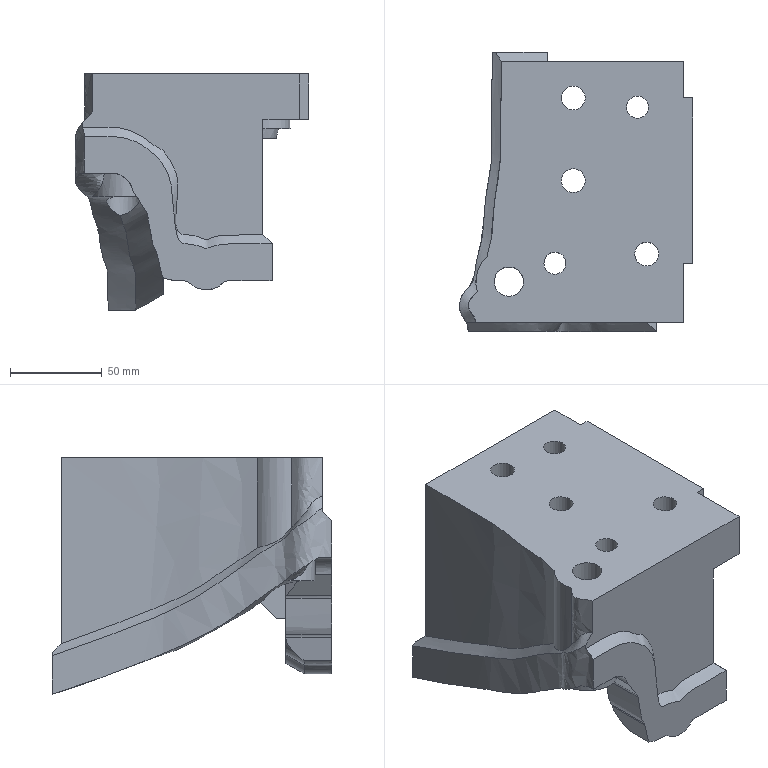Part | NX | features solid 2 | 1 solid | 74 faces | box 126.997 x 151.993 x 128.695 mm | volume 839297 mm3 | plane 38 | cylinder 19 | spline 14 | cone 3 | commonest cylinder face diameters 13 x5 32 x4 36 x3 10 x2 12 x2 16 x1